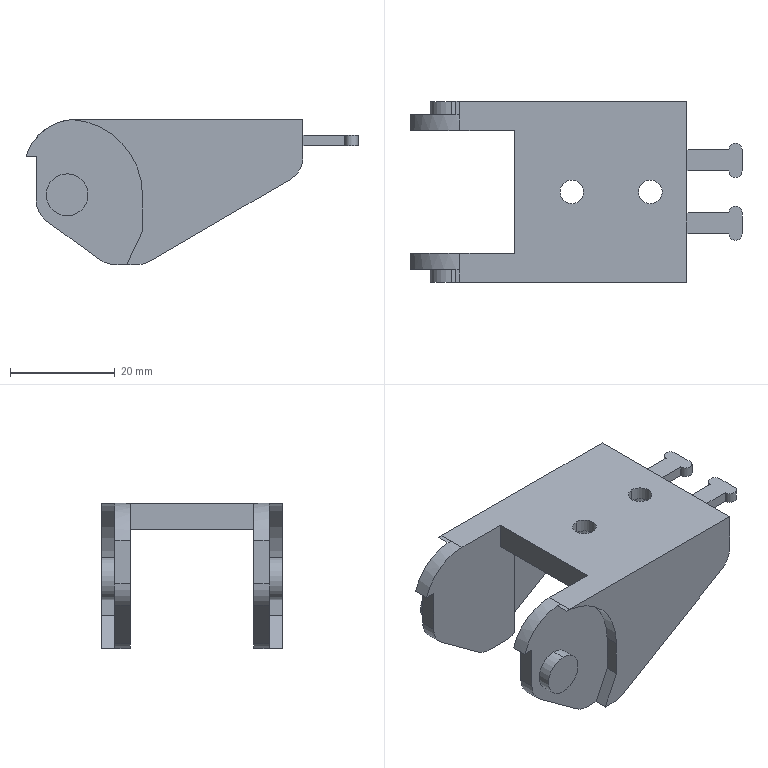Part | NX | features BREP 1 | 1 solid | 66 faces | box 63.364 x 34.5 x 27.7 mm | volume 11296 mm3 | plane 38 | cylinder 24 | cone 4 | commonest cylinder face diameters 10 x8 2.5 x4 4.5 x4 8 x4 20 x2 28.749 x2